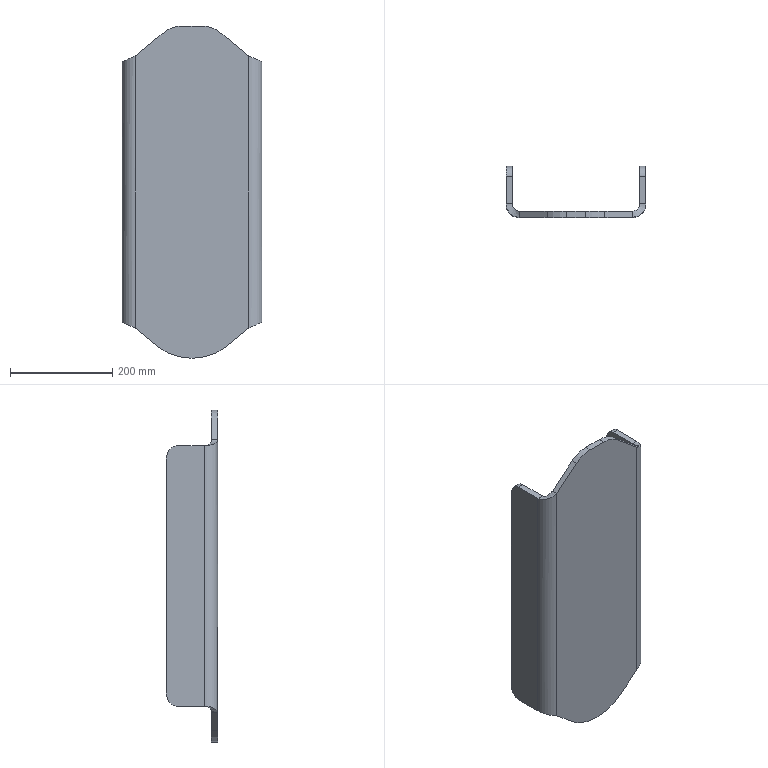Part | SolidWorks | features Fillet 3, Extrusion 1, FlatPattern 1, ICE 1, SheetMetal 1, SolidToSheetMetal 1 | 1 solid | 34 faces | box 274 x 100 x 650 mm | volume 2917891 mm3 | plane 18 | spline 8 | cylinder 8 | commonest cylinder face diameters 28 x2 52 x2 120 x2 200 x2
STEP:
#1=CARTESIAN_POINT('',(137.,-57.,579.897));
#2=VERTEX_POINT('',#1);
#3=CARTESIAN_POINT('',(125.,-57.,579.897));
#4=VERTEX_POINT('',#3);
#5=CARTESIAN_POINT('',(125.,-57.,579.897));
#6=DIRECTION('',(-1.,0.,0.));
#7=VECTOR('',#6,1000.);
#8=LINE('',#5,#7);
#9=EDGE_CURVE('',#2,#4,#8,.T.);
#10=ORIENTED_EDGE('',*,*,#9,.F.);
#11=CARTESIAN_POINT('',(137.,-37.,553.972));
#12=VERTEX_POINT('',#11);
#13=CARTESIAN_POINT('',(137.,-57.,579.897));
#14=CARTESIAN_POINT('',(137.,-45.284,579.897));
#15=CARTESIAN_POINT('',(137.,-37.,569.159));
#16=CARTESIAN_POINT('',(137.,-37.,553.972));
#17=(BOUNDED_CURVE()B_SPLINE_CURVE(3,(#13,#14,#15,#16),.UNSPECIFIED.,.F.,.F.)B_SPLINE_CURVE_WITH_KNOTS((4,4),(3.142,4.712),.UNSPECIFIED.)CURVE()GEOMETRIC_REPRESENTATION_ITEM()RATIONAL_B_SPLINE_CURVE((1.,0.8047,0.8047,1.))REPRESENTATION_ITEM(''));
#18=EDGE_CURVE('',#2,#12,#17,.T.);
#19=ORIENTED_EDGE('',*,*,#18,.T.);
#20=CARTESIAN_POINT('',(125.,-37.,553.972));
#21=VERTEX_POINT('',#20);
#22=CARTESIAN_POINT('',(125.,-37.,553.972));
#23=DIRECTION('',(-1.,0.,0.));
#24=VECTOR('',#23,1000.);
#25=LINE('',#22,#24);
#26=EDGE_CURVE('',#12,#21,#25,.T.);
#27=ORIENTED_EDGE('',*,*,#26,.T.);
#28=CARTESIAN_POINT('',(125.,-57.,579.897));
#29=CARTESIAN_POINT('',(125.,-45.284,579.897));
#30=CARTESIAN_POINT('',(125.,-37.,569.159));
#31=CARTESIAN_POINT('',(125.,-37.,553.972));
#32=(BOUNDED_CURVE()B_SPLINE_CURVE(3,(#28,#29,#30,#31),.UNSPECIFIED.,.F.,.T.)B_SPLINE_CURVE_WITH_KNOTS((4,4),(3.142,4.712),.UNSPECIFIED.)CURVE()GEOMETRIC_REPRESENTATION_ITEM()RATIONAL_B_SPLINE_CURVE((1.,0.8047,0.8047,1.))REPRESENTATION_ITEM(''));
#33=EDGE_CURVE('',#4,#21,#32,.T.);
#34=ORIENTED_EDGE('',*,*,#33,.F.);
#35=EDGE_LOOP('',(#10,#19,#27,#34));
#36=FACE_OUTER_BOUND('',#35,.T.);
#37=CARTESIAN_POINT('',(125.,-37.,553.972));
#38=CARTESIAN_POINT('',(137.,-37.,553.972));
#39=CARTESIAN_POINT('',(125.,-37.,569.159));
#40=CARTESIAN_POINT('',(137.,-37.,569.159));
#41=CARTESIAN_POINT('',(125.,-45.284,579.897));
#42=CARTESIAN_POINT('',(137.,-45.284,579.897));
#43=CARTESIAN_POINT('',(125.,-57.,579.897));
#44=CARTESIAN_POINT('',(137.,-57.,579.897));
#45=(BOUNDED_SURFACE()B_SPLINE_SURFACE(3,1,((#37,#38),(#39,#40),(#41,#42),(#43,#44)),.UNSPECIFIED.,.F.,.F.,.F.)B_SPLINE_SURFACE_WITH_KNOTS((4,4),(2,2),(0.,1.),(0.,1.),.UNSPECIFIED.)GEOMETRIC_REPRESENTATION_ITEM()RATIONAL_B_SPLINE_SURFACE(((1.,1.),(0.8047,0.8047),(0.8047,0.8047),(1.,1.)))REPRESENTATION_ITEM('')SURFACE());
#46=ADVANCED_FACE('',(#36),#45,.T.);
#47=ORIENTED_EDGE('',*,*,#26,.F.);
#48=CARTESIAN_POINT('',(137.,-37.,96.028));
#49=VERTEX_POINT('',#48);
#50=CARTESIAN_POINT('',(137.,-37.,650.));
#51=DIRECTION('',(0.,0.,-1.));
#52=VECTOR('',#51,1000.);
#53=LINE('',#50,#52);
#54=EDGE_CURVE('',#12,#49,#53,.T.);
#55=ORIENTED_EDGE('',*,*,#54,.T.);
#56=CARTESIAN_POINT('',(125.,-37.,96.028));
#57=VERTEX_POINT('',#56);
#58=CARTESIAN_POINT('',(125.,-37.,96.028));
#59=DIRECTION('',(-1.,0.,0.));
#60=VECTOR('',#59,1000.);
#61=LINE('',#58,#60);
#62=EDGE_CURVE('',#49,#57,#61,.T.);
#63=ORIENTED_EDGE('',*,*,#62,.T.);
#64=CARTESIAN_POINT('',(125.,-37.,650.));
#65=DIRECTION('',(0.,0.,-1.));
#66=VECTOR('',#65,1000.);
#67=LINE('',#64,#66);
#68=EDGE_CURVE('',#21,#57,#67,.T.);
#69=ORIENTED_EDGE('',*,*,#68,.F.);
#70=EDGE_LOOP('',(#47,#55,#63,#69));
#71=FACE_OUTER_BOUND('',#70,.T.);
#72=CARTESIAN_POINT('',(125.,-37.,650.));
#73=DIRECTION('',(0.,-1.,0.));
#74=DIRECTION('',(0.,0.,-1.));
#75=AXIS2_PLACEMENT_3D('',#72,#73,#74);
#76=PLANE('',#75);
#77=ADVANCED_FACE('',(#71),#76,.F.);
#78=ORIENTED_EDGE('',*,*,#62,.F.);
#79=CARTESIAN_POINT('',(137.,-57.,70.103));
#80=VERTEX_POINT('',#79);
#81=CARTESIAN_POINT('',(137.,-37.,96.028));
#82=CARTESIAN_POINT('',(137.,-37.,80.841));
#83=CARTESIAN_POINT('',(137.,-45.284,70.103));
#84=CARTESIAN_POINT('',(137.,-57.,70.103));
#85=(BOUNDED_CURVE()B_SPLINE_CURVE(3,(#81,#82,#83,#84),.UNSPECIFIED.,.F.,.F.)B_SPLINE_CURVE_WITH_KNOTS((4,4),(4.712,6.283),.UNSPECIFIED.)CURVE()GEOMETRIC_REPRESENTATION_ITEM()RATIONAL_B_SPLINE_CURVE((1.,0.8047,0.8047,1.))REPRESENTATION_ITEM(''));
#86=EDGE_CURVE('',#49,#80,#85,.T.);
#87=ORIENTED_EDGE('',*,*,#86,.T.);
#88=CARTESIAN_POINT('',(125.,-57.,70.103));
#89=VERTEX_POINT('',#88);
#90=CARTESIAN_POINT('',(125.,-57.,70.103));
#91=DIRECTION('',(-1.,0.,0.));
#92=VECTOR('',#91,1000.);
#93=LINE('',#90,#92);
#94=EDGE_CURVE('',#80,#89,#93,.T.);
#95=ORIENTED_EDGE('',*,*,#94,.T.);
#96=CARTESIAN_POINT('',(125.,-37.,96.028));
#97=CARTESIAN_POINT('',(125.,-37.,80.841));
#98=CARTESIAN_POINT('',(125.,-45.284,70.103));
#99=CARTESIAN_POINT('',(125.,-57.,70.103));
#100=(BOUNDED_CURVE()B_SPLINE_CURVE(3,(#96,#97,#98,#99),.UNSPECIFIED.,.F.,.T.)B_SPLINE_CURVE_WITH_KNOTS((4,4),(4.712,6.283),.UNSPECIFIED.)CURVE()GEOMETRIC_REPRESENTATION_ITEM()RATIONAL_B_SPLINE_CURVE((1.,0.8047,0.8047,1.))REPRESENTATION_ITEM(''));
#101=EDGE_CURVE('',#57,#89,#100,.T.);
#102=ORIENTED_EDGE('',*,*,#101,.F.);
#103=EDGE_LOOP('',(#78,#87,#95,#102));
#104=FACE_OUTER_BOUND('',#103,.T.);
#105=CARTESIAN_POINT('',(125.,-57.,70.103));
#106=CARTESIAN_POINT('',(137.,-57.,70.103));
#107=CARTESIAN_POINT('',(125.,-45.284,70.103));
#108=CARTESIAN_POINT('',(137.,-45.284,70.103));
#109=CARTESIAN_POINT('',(125.,-37.,80.841));
#110=CARTESIAN_POINT('',(137.,-37.,80.841));
#111=CARTESIAN_POINT('',(125.,-37.,96.028));
#112=CARTESIAN_POINT('',(137.,-37.,96.028));
#113=(BOUNDED_SURFACE()B_SPLINE_SURFACE(3,1,((#105,#106),(#107,#108),(#109,#110),(#111,#112)),.UNSPECIFIED.,.F.,.F.,.F.)B_SPLINE_SURFACE_WITH_KNOTS((4,4),(2,2),(0.,1.),(0.,1.),.UNSPECIFIED.)GEOMETRIC_REPRESENTATION_ITEM()RATIONAL_B_SPLINE_SURFACE(((1.,1.),(0.8047,0.8047),(0.8047,0.8047),(1.,1.)))REPRESENTATION_ITEM('')SURFACE());
#114=ADVANCED_FACE('',(#104),#113,.T.);
#115=ORIENTED_EDGE('',*,*,#94,.F.);
#116=CARTESIAN_POINT('',(137.,-111.,70.103));
#117=VERTEX_POINT('',#116);
#118=CARTESIAN_POINT('',(137.,-37.,70.103));
#119=DIRECTION('',(0.,-1.,0.));
#120=VECTOR('',#119,1000.);
#121=LINE('',#118,#120);
#122=EDGE_CURVE('',#80,#117,#121,.T.);
#123=ORIENTED_EDGE('',*,*,#122,.T.);
#124=CARTESIAN_POINT('',(125.,-111.,70.103));
#125=VERTEX_POINT('',#124);
#126=CARTESIAN_POINT('',(125.,-111.,70.103));
#127=DIRECTION('',(-1.,0.,0.));
#128=VECTOR('',#127,1000.);
#129=LINE('',#126,#128);
#130=EDGE_CURVE('',#117,#125,#129,.T.);
#131=ORIENTED_EDGE('',*,*,#130,.T.);
#132=CARTESIAN_POINT('',(125.,-37.,70.103));
#133=DIRECTION('',(0.,-1.,0.));
#134=VECTOR('',#133,1000.);
#135=LINE('',#132,#134);
#136=EDGE_CURVE('',#89,#125,#135,.T.);
#137=ORIENTED_EDGE('',*,*,#136,.F.);
#138=EDGE_LOOP('',(#115,#123,#131,#137));
#139=FACE_OUTER_BOUND('',#138,.T.);
#140=CARTESIAN_POINT('',(125.,-37.,70.103));
#141=DIRECTION('',(0.,0.,1.));
#142=DIRECTION('',(0.,-1.,0.));
#143=AXIS2_PLACEMENT_3D('',#140,#141,#142);
#144=PLANE('',#143);
#145=ADVANCED_FACE('',(#139),#144,.F.);
#146=ORIENTED_EDGE('',*,*,#130,.F.);
#147=CARTESIAN_POINT('',(111.,-137.,58.557));
#148=VERTEX_POINT('',#147);
#149=CARTESIAN_POINT('',(137.,-111.,70.103));
#150=CARTESIAN_POINT('',(137.,-126.23,70.103));
#151=CARTESIAN_POINT('',(126.23,-137.,65.32));
#152=CARTESIAN_POINT('',(111.,-137.,58.557));
#153=(BOUNDED_CURVE()B_SPLINE_CURVE(3,(#149,#150,#151,#152),.UNSPECIFIED.,.F.,.F.)B_SPLINE_CURVE_WITH_KNOTS((4,4),(3.142,4.712),.UNSPECIFIED.)CURVE()GEOMETRIC_REPRESENTATION_ITEM()RATIONAL_B_SPLINE_CURVE((1.,0.8047,0.8047,1.))REPRESENTATION_ITEM(''));
#154=EDGE_CURVE('',#117,#148,#153,.T.);
#155=ORIENTED_EDGE('',*,*,#154,.T.);
#156=CARTESIAN_POINT('',(111.,-125.,58.557));
#157=VERTEX_POINT('',#156);
#158=CARTESIAN_POINT('',(111.,-125.,58.557));
#159=DIRECTION('',(0.,1.,0.));
#160=VECTOR('',#159,1000.);
#161=LINE('',#158,#160);
#162=EDGE_CURVE('',#148,#157,#161,.T.);
#163=ORIENTED_EDGE('',*,*,#162,.T.);
#164=CARTESIAN_POINT('',(125.,-111.,70.103));
#165=CARTESIAN_POINT('',(125.,-119.201,70.103));
#166=CARTESIAN_POINT('',(119.201,-125.,65.32));
#167=CARTESIAN_POINT('',(111.,-125.,58.557));
#168=(BOUNDED_CURVE()B_SPLINE_CURVE(3,(#164,#165,#166,#167),.UNSPECIFIED.,.F.,.F.)B_SPLINE_CURVE_WITH_KNOTS((4,4),(3.142,4.712),.UNSPECIFIED.)CURVE()GEOMETRIC_REPRESENTATION_ITEM()RATIONAL_B_SPLINE_CURVE((1.,0.8047,0.8047,1.))REPRESENTATION_ITEM(''));
#169=EDGE_CURVE('',#125,#157,#168,.T.);
#170=ORIENTED_EDGE('',*,*,#169,.F.);
#171=EDGE_LOOP('',(#146,#155,#163,#170));
#172=FACE_OUTER_BOUND('',#171,.T.);
#173=CARTESIAN_POINT('',(85.,-111.,47.01));
#174=CARTESIAN_POINT('',(89.,-111.,47.01));
#175=CARTESIAN_POINT('',(93.,-111.,47.01));
#176=CARTESIAN_POINT('',(97.,-111.,47.01));
#177=CARTESIAN_POINT('',(85.,-59.,47.01));
#178=CARTESIAN_POINT('',(89.,-67.,47.01));
#179=CARTESIAN_POINT('',(93.,-75.,47.01));
#180=CARTESIAN_POINT('',(97.,-83.,47.01));
#181=CARTESIAN_POINT('',(137.,-59.,70.103));
#182=CARTESIAN_POINT('',(133.,-67.,70.103));
#183=CARTESIAN_POINT('',(129.,-75.,70.103));
#184=CARTESIAN_POINT('',(125.,-83.,70.103));
#185=CARTESIAN_POINT('',(137.,-111.,70.103));
#186=CARTESIAN_POINT('',(133.,-111.,70.103));
#187=CARTESIAN_POINT('',(129.,-111.,70.103));
#188=CARTESIAN_POINT('',(125.,-111.,70.103));
#189=CARTESIAN_POINT('',(137.,-163.,70.103));
#190=CARTESIAN_POINT('',(133.,-155.,70.103));
#191=CARTESIAN_POINT('',(129.,-147.,70.103));
#192=CARTESIAN_POINT('',(125.,-139.,70.103));
#193=CARTESIAN_POINT('',(85.,-163.,47.01));
#194=CARTESIAN_POINT('',(89.,-155.,47.01));
#195=CARTESIAN_POINT('',(93.,-147.,47.01));
#196=CARTESIAN_POINT('',(97.,-139.,47.01));
#197=CARTESIAN_POINT('',(85.,-111.,47.01));
#198=CARTESIAN_POINT('',(89.,-111.,47.01));
#199=CARTESIAN_POINT('',(93.,-111.,47.01));
#200=CARTESIAN_POINT('',(97.,-111.,47.01));
#201=(BOUNDED_SURFACE()B_SPLINE_SURFACE(3,3,((#173,#174,#175,#176),(#177,#178,#179,#180),(#181,#182,#183,#184),(#185,#186,#187,#188),(#189,#190,#191,#192),(#193,#194,#195,#196),(#197,#198,#199,#200)),.UNSPECIFIED.,.T.,.F.,.F.)B_SPLINE_SURFACE_WITH_KNOTS((4,3,4),(4,4),(0.,0.5,1.),(0.,1.),.UNSPECIFIED.)GEOMETRIC_REPRESENTATION_ITEM()RATIONAL_B_SPLINE_SURFACE(((1.,1.,1.,1.),(0.3333,0.3333,0.3333,0.3333),(0.3333,0.3333,0.3333,0.3333),(1.,1.,1.,1.),(0.3333,0.3333,0.3333,0.3333),(0.3333,0.3333,0.3333,0.3333),(1.,1.,1.,1.)))REPRESENTATION_ITEM('')SURFACE());
#202=ADVANCED_FACE('',(#172),#201,.T.);
#203=ORIENTED_EDGE('',*,*,#162,.F.);
#204=CARTESIAN_POINT('',(67.709,-137.,22.853));
#205=VERTEX_POINT('',#204);
#206=CARTESIAN_POINT('',(269.189,-137.,189.021));
#207=DIRECTION('',(-0.7715,0.,-0.6363));
#208=VECTOR('',#207,1000.);
#209=LINE('',#206,#208);
#210=EDGE_CURVE('',#148,#205,#209,.T.);
#211=ORIENTED_EDGE('',*,*,#210,.T.);
#212=CARTESIAN_POINT('',(67.709,-125.,22.853));
#213=VERTEX_POINT('',#212);
#214=CARTESIAN_POINT('',(67.709,-125.,22.853));
#215=DIRECTION('',(0.,1.,0.));
#216=VECTOR('',#215,1000.);
#217=LINE('',#214,#216);
#218=EDGE_CURVE('',#205,#213,#217,.T.);
#219=ORIENTED_EDGE('',*,*,#218,.T.);
#220=CARTESIAN_POINT('',(269.189,-125.,189.021));
#221=DIRECTION('',(-0.7715,0.,-0.6363));
#222=VECTOR('',#221,1000.);
#223=LINE('',#220,#222);
#224=EDGE_CURVE('',#157,#213,#223,.T.);
#225=ORIENTED_EDGE('',*,*,#224,.F.);
#226=EDGE_LOOP('',(#203,#211,#219,#225));
#227=FACE_OUTER_BOUND('',#226,.T.);
#228=CARTESIAN_POINT('',(269.189,-125.,189.021));
#229=DIRECTION('',(-0.6363,0.,0.7715));
#230=DIRECTION('',(-0.7715,0.,-0.6363));
#231=AXIS2_PLACEMENT_3D('',#228,#229,#230);
#232=PLANE('',#231);
#233=ADVANCED_FACE('',(#227),#232,.F.);
#234=ORIENTED_EDGE('',*,*,#218,.F.);
#235=CARTESIAN_POINT('',(4.083,-137.,0.));
#236=VERTEX_POINT('',#235);
#237=CARTESIAN_POINT('',(4.083,-137.,100.));
#238=DIRECTION('',(0.,1.,0.));
#239=DIRECTION('',(1.,0.,0.));
#240=AXIS2_PLACEMENT_3D('',#237,#238,#239);
#241=CIRCLE('',#240,100.);
#242=EDGE_CURVE('',#205,#236,#241,.T.);
#243=ORIENTED_EDGE('',*,*,#242,.T.);
#244=CARTESIAN_POINT('',(4.083,-125.,0.));
#245=VERTEX_POINT('',#244);
#246=CARTESIAN_POINT('',(4.083,-125.,0.));
#247=DIRECTION('',(0.,1.,0.));
#248=VECTOR('',#247,1000.);
#249=LINE('',#246,#248);
#250=EDGE_CURVE('',#236,#245,#249,.T.);
#251=ORIENTED_EDGE('',*,*,#250,.T.);
#252=CARTESIAN_POINT('',(4.083,-125.,100.));
#253=DIRECTION('',(0.,1.,0.));
#254=DIRECTION('',(1.,0.,0.));
#255=AXIS2_PLACEMENT_3D('',#252,#253,#254);
#256=CIRCLE('',#255,100.);
#257=EDGE_CURVE('',#213,#245,#256,.T.);
#258=ORIENTED_EDGE('',*,*,#257,.F.);
#259=EDGE_LOOP('',(#234,#243,#251,#258));
#260=FACE_OUTER_BOUND('',#259,.T.);
#261=CARTESIAN_POINT('',(4.083,-125.,100.));
#262=DIRECTION('',(0.,-1.,0.));
#263=DIRECTION('',(1.,0.,0.));
#264=AXIS2_PLACEMENT_3D('',#261,#262,#263);
#265=CYLINDRICAL_SURFACE('',#264,100.);
#266=ADVANCED_FACE('',(#260),#265,.T.);
#267=ORIENTED_EDGE('',*,*,#250,.F.);
#268=CARTESIAN_POINT('',(-4.083,-137.,0.));
#269=VERTEX_POINT('',#268);
#270=CARTESIAN_POINT('',(-111.,-137.,0.));
#271=DIRECTION('',(-1.,0.,0.));
#272=VECTOR('',#271,1000.);
#273=LINE('',#270,#272);
#274=EDGE_CURVE('',#236,#269,#273,.T.);
#275=ORIENTED_EDGE('',*,*,#274,.T.);
#276=CARTESIAN_POINT('',(-4.083,-125.,0.));
#277=VERTEX_POINT('',#276);
#278=CARTESIAN_POINT('',(-4.083,-125.,0.));
#279=DIRECTION('',(0.,1.,0.));
#280=VECTOR('',#279,1000.);
#281=LINE('',#278,#280);
#282=EDGE_CURVE('',#269,#277,#281,.T.);
#283=ORIENTED_EDGE('',*,*,#282,.T.);
#284=CARTESIAN_POINT('',(-111.,-125.,0.));
#285=DIRECTION('',(-1.,0.,0.));
#286=VECTOR('',#285,1000.);
#287=LINE('',#284,#286);
#288=EDGE_CURVE('',#245,#277,#287,.T.);
#289=ORIENTED_EDGE('',*,*,#288,.F.);
#290=EDGE_LOOP('',(#267,#275,#283,#289));
#291=FACE_OUTER_BOUND('',#290,.T.);
#292=CARTESIAN_POINT('',(-111.,-125.,0.));
#293=DIRECTION('',(0.,0.,1.));
#294=DIRECTION('',(-1.,0.,0.));
#295=AXIS2_PLACEMENT_3D('',#292,#293,#294);
#296=PLANE('',#295);
#297=ADVANCED_FACE('',(#291),#296,.F.);
#298=ORIENTED_EDGE('',*,*,#282,.F.);
#299=CARTESIAN_POINT('',(-67.709,-137.,22.853));
#300=VERTEX_POINT('',#299);
#301=CARTESIAN_POINT('',(-4.083,-137.,100.));
#302=DIRECTION('',(0.,1.,0.));
#303=DIRECTION('',(1.,0.,0.));
#304=AXIS2_PLACEMENT_3D('',#301,#302,#303);
#305=CIRCLE('',#304,100.);
#306=EDGE_CURVE('',#269,#300,#305,.T.);
#307=ORIENTED_EDGE('',*,*,#306,.T.);
#308=CARTESIAN_POINT('',(-67.709,-125.,22.853));
#309=VERTEX_POINT('',#308);
#310=CARTESIAN_POINT('',(-67.709,-125.,22.853));
#311=DIRECTION('',(0.,1.,0.));
#312=VECTOR('',#311,1000.);
#313=LINE('',#310,#312);
#314=EDGE_CURVE('',#300,#309,#313,.T.);
#315=ORIENTED_EDGE('',*,*,#314,.T.);
#316=CARTESIAN_POINT('',(-4.083,-125.,100.));
#317=DIRECTION('',(0.,1.,0.));
#318=DIRECTION('',(1.,0.,0.));
#319=AXIS2_PLACEMENT_3D('',#316,#317,#318);
#320=CIRCLE('',#319,100.);
#321=EDGE_CURVE('',#277,#309,#320,.T.);
#322=ORIENTED_EDGE('',*,*,#321,.F.);
#323=EDGE_LOOP('',(#298,#307,#315,#322));
#324=FACE_OUTER_BOUND('',#323,.T.);
#325=CARTESIAN_POINT('',(-4.083,-125.,100.));
#326=DIRECTION('',(0.,-1.,0.));
#327=DIRECTION('',(1.,0.,0.));
#328=AXIS2_PLACEMENT_3D('',#325,#326,#327);
#329=CYLINDRICAL_SURFACE('',#328,100.);
#330=ADVANCED_FACE('',(#324),#329,.T.);
#331=ORIENTED_EDGE('',*,*,#314,.F.);
#332=CARTESIAN_POINT('',(-111.,-137.,58.557));
#333=VERTEX_POINT('',#332);
#334=CARTESIAN_POINT('',(-401.316,-137.,297.992));
#335=DIRECTION('',(-0.7715,0.,0.6363));
#336=VECTOR('',#335,1000.);
#337=LINE('',#334,#336);
#338=EDGE_CURVE('',#300,#333,#337,.T.);
#339=ORIENTED_EDGE('',*,*,#338,.T.);
#340=CARTESIAN_POINT('',(-111.,-125.,58.557));
#341=VERTEX_POINT('',#340);
#342=CARTESIAN_POINT('',(-111.,-125.,58.557));
#343=DIRECTION('',(0.,1.,0.));
#344=VECTOR('',#343,1000.);
#345=LINE('',#342,#344);
#346=EDGE_CURVE('',#333,#341,#345,.T.);
#347=ORIENTED_EDGE('',*,*,#346,.T.);
#348=CARTESIAN_POINT('',(-401.316,-125.,297.992));
#349=DIRECTION('',(-0.7715,0.,0.6363));
#350=VECTOR('',#349,1000.);
#351=LINE('',#348,#350);
#352=EDGE_CURVE('',#309,#341,#351,.T.);
#353=ORIENTED_EDGE('',*,*,#352,.F.);
#354=EDGE_LOOP('',(#331,#339,#347,#353));
#355=FACE_OUTER_BOUND('',#354,.T.);
#356=CARTESIAN_POINT('',(-401.316,-125.,297.992));
#357=DIRECTION('',(0.6363,0.,0.7715));
#358=DIRECTION('',(-0.7715,0.,0.6363));
#359=AXIS2_PLACEMENT_3D('',#356,#357,#358);
#360=PLANE('',#359);
#361=ADVANCED_FACE('',(#355),#360,.F.);
#362=ORIENTED_EDGE('',*,*,#346,.F.);
#363=CARTESIAN_POINT('',(-137.,-111.,70.103));
#364=VERTEX_POINT('',#363);
#365=CARTESIAN_POINT('',(-111.,-137.,58.557));
#366=CARTESIAN_POINT('',(-126.23,-137.,65.32));
#367=CARTESIAN_POINT('',(-137.,-126.23,70.103));
#368=CARTESIAN_POINT('',(-137.,-111.,70.103));
#369=(BOUNDED_CURVE()B_SPLINE_CURVE(3,(#365,#366,#367,#368),.UNSPECIFIED.,.F.,.T.)B_SPLINE_CURVE_WITH_KNOTS((4,4),(1.571,3.142),.UNSPECIFIED.)CURVE()GEOMETRIC_REPRESENTATION_ITEM()RATIONAL_B_SPLINE_CURVE((1.,0.8047,0.8047,1.))REPRESENTATION_ITEM(''));
#370=EDGE_CURVE('',#333,#364,#369,.T.);
#371=ORIENTED_EDGE('',*,*,#370,.T.);
#372=CARTESIAN_POINT('',(-125.,-111.,70.103));
#373=VERTEX_POINT('',#372);
#374=CARTESIAN_POINT('',(-125.,-111.,70.103));
#375=DIRECTION('',(1.,0.,0.));
#376=VECTOR('',#375,1000.);
#377=LINE('',#374,#376);
#378=EDGE_CURVE('',#364,#373,#377,.T.);
#379=ORIENTED_EDGE('',*,*,#378,.T.);
#380=CARTESIAN_POINT('',(-111.,-125.,58.557));
#381=CARTESIAN_POINT('',(-119.201,-125.,65.32));
#382=CARTESIAN_POINT('',(-125.,-119.201,70.103));
#383=CARTESIAN_POINT('',(-125.,-111.,70.103));
#384=(BOUNDED_CURVE()B_SPLINE_CURVE(3,(#380,#381,#382,#383),.UNSPECIFIED.,.F.,.T.)B_SPLINE_CURVE_WITH_KNOTS((4,4),(1.571,3.142),.UNSPECIFIED.)CURVE()GEOMETRIC_REPRESENTATION_ITEM()RATIONAL_B_SPLINE_CURVE((1.,0.8047,0.8047,1.))REPRESENTATION_ITEM(''));
#385=EDGE_CURVE('',#341,#373,#384,.T.);
#386=ORIENTED_EDGE('',*,*,#385,.F.);
#387=EDGE_LOOP('',(#362,#371,#379,#386));
#388=FACE_OUTER_BOUND('',#387,.T.);
#389=CARTESIAN_POINT('',(-85.,-111.,47.01));
#390=CARTESIAN_POINT('',(-89.,-111.,47.01));
#391=CARTESIAN_POINT('',(-93.,-111.,47.01));
#392=CARTESIAN_POINT('',(-97.,-111.,47.01));
#393=CARTESIAN_POINT('',(-85.,-163.,47.01));
#394=CARTESIAN_POINT('',(-89.,-155.,47.01));
#395=CARTESIAN_POINT('',(-93.,-147.,47.01));
#396=CARTESIAN_POINT('',(-97.,-139.,47.01));
#397=CARTESIAN_POINT('',(-137.,-163.,70.103));
#398=CARTESIAN_POINT('',(-133.,-155.,70.103));
#399=CARTESIAN_POINT('',(-129.,-147.,70.103));
#400=CARTESIAN_POINT('',(-125.,-139.,70.103));
#401=CARTESIAN_POINT('',(-137.,-111.,70.103));
#402=CARTESIAN_POINT('',(-133.,-111.,70.103));
#403=CARTESIAN_POINT('',(-129.,-111.,70.103));
#404=CARTESIAN_POINT('',(-125.,-111.,70.103));
#405=CARTESIAN_POINT('',(-137.,-59.,70.103));
#406=CARTESIAN_POINT('',(-133.,-67.,70.103));
#407=CARTESIAN_POINT('',(-129.,-75.,70.103));
#408=CARTESIAN_POINT('',(-125.,-83.,70.103));
#409=CARTESIAN_POINT('',(-85.,-59.,47.01));
#410=CARTESIAN_POINT('',(-89.,-67.,47.01));
#411=CARTESIAN_POINT('',(-93.,-75.,47.01));
#412=CARTESIAN_POINT('',(-97.,-83.,47.01));
#413=CARTESIAN_POINT('',(-85.,-111.,47.01));
#414=CARTESIAN_POINT('',(-89.,-111.,47.01));
#415=CARTESIAN_POINT('',(-93.,-111.,47.01));
#416=CARTESIAN_POINT('',(-97.,-111.,47.01));
#417=(BOUNDED_SURFACE()B_SPLINE_SURFACE(3,3,((#389,#390,#391,#392),(#393,#394,#395,#396),(#397,#398,#399,#400),(#401,#402,#403,#404),(#405,#406,#407,#408),(#409,#410,#411,#412),(#413,#414,#415,#416)),.UNSPECIFIED.,.T.,.F.,.F.)B_SPLINE_SURFACE_WITH_KNOTS((4,3,4),(4,4),(0.,0.5,1.),(0.,1.),.UNSPECIFIED.)GEOMETRIC_REPRESENTATION_ITEM()RATIONAL_B_SPLINE_SURFACE(((1.,1.,1.,1.),(0.3333,0.3333,0.3333,0.3333),(0.3333,0.3333,0.3333,0.3333),(1.,1.,1.,1.),(0.3333,0.3333,0.3333,0.3333),(0.3333,0.3333,0.3333,0.3333),(1.,1.,1.,1.)))REPRESENTATION_ITEM('')SURFACE());
#418=ADVANCED_FACE('',(#388),#417,.T.);
#419=ORIENTED_EDGE('',*,*,#378,.F.);
#420=CARTESIAN_POINT('',(-137.,-57.,70.103));
#421=VERTEX_POINT('',#420);
#422=CARTESIAN_POINT('',(-137.,-37.,70.103));
#423=DIRECTION('',(0.,1.,0.));
#424=VECTOR('',#423,1000.);
#425=LINE('',#422,#424);
#426=EDGE_CURVE('',#364,#421,#425,.T.);
#427=ORIENTED_EDGE('',*,*,#426,.T.);
#428=CARTESIAN_POINT('',(-125.,-57.,70.103));
#429=VERTEX_POINT('',#428);
#430=CARTESIAN_POINT('',(-125.,-57.,70.103));
#431=DIRECTION('',(1.,0.,0.));
#432=VECTOR('',#431,1000.);
#433=LINE('',#430,#432);
#434=EDGE_CURVE('',#421,#429,#433,.T.);
#435=ORIENTED_EDGE('',*,*,#434,.T.);
#436=CARTESIAN_POINT('',(-125.,-37.,70.103));
#437=DIRECTION('',(0.,1.,0.));
#438=VECTOR('',#437,1000.);
#439=LINE('',#436,#438);
#440=EDGE_CURVE('',#373,#429,#439,.T.);
#441=ORIENTED_EDGE('',*,*,#440,.F.);
#442=EDGE_LOOP('',(#419,#427,#435,#441));
#443=FACE_OUTER_BOUND('',#442,.T.);
#444=CARTESIAN_POINT('',(-125.,-37.,70.103));
#445=DIRECTION('',(0.,0.,1.));
#446=DIRECTION('',(0.,1.,0.));
#447=AXIS2_PLACEMENT_3D('',#444,#445,#446);
#448=PLANE('',#447);
#449=ADVANCED_FACE('',(#443),#448,.F.);
#450=ORIENTED_EDGE('',*,*,#434,.F.);
#451=CARTESIAN_POINT('',(-137.,-37.,96.028));
#452=VERTEX_POINT('',#451);
#453=CARTESIAN_POINT('',(-137.,-57.,70.103));
#454=CARTESIAN_POINT('',(-137.,-45.284,70.103));
#455=CARTESIAN_POINT('',(-137.,-37.,80.841));
#456=CARTESIAN_POINT('',(-137.,-37.,96.028));
#457=(BOUNDED_CURVE()B_SPLINE_CURVE(3,(#453,#454,#455,#456),.UNSPECIFIED.,.F.,.T.)B_SPLINE_CURVE_WITH_KNOTS((4,4),(3.142,4.712),.UNSPECIFIED.)CURVE()GEOMETRIC_REPRESENTATION_ITEM()RATIONAL_B_SPLINE_CURVE((1.,0.8047,0.8047,1.))REPRESENTATION_ITEM(''));
#458=EDGE_CURVE('',#421,#452,#457,.T.);
#459=ORIENTED_EDGE('',*,*,#458,.T.);
#460=CARTESIAN_POINT('',(-125.,-37.,96.028));
#461=VERTEX_POINT('',#460);
#462=CARTESIAN_POINT('',(-125.,-37.,96.028));
#463=DIRECTION('',(1.,0.,0.));
#464=VECTOR('',#463,1000.);
#465=LINE('',#462,#464);
#466=EDGE_CURVE('',#452,#461,#465,.T.);
#467=ORIENTED_EDGE('',*,*,#466,.T.);
#468=CARTESIAN_POINT('',(-125.,-57.,70.103));
#469=CARTESIAN_POINT('',(-125.,-45.284,70.103));
#470=CARTESIAN_POINT('',(-125.,-37.,80.841));
#471=CARTESIAN_POINT('',(-125.,-37.,96.028));
#472=(BOUNDED_CURVE()B_SPLINE_CURVE(3,(#468,#469,#470,#471),.UNSPECIFIED.,.F.,.F.)B_SPLINE_CURVE_WITH_KNOTS((4,4),(3.142,4.712),.UNSPECIFIED.)CURVE()GEOMETRIC_REPRESENTATION_ITEM()RATIONAL_B_SPLINE_CURVE((1.,0.8047,0.8047,1.))REPRESENTATION_ITEM(''));
#473=EDGE_CURVE('',#429,#461,#472,.T.);
#474=ORIENTED_EDGE('',*,*,#473,.F.);
#475=EDGE_LOOP('',(#450,#459,#467,#474));
#476=FACE_OUTER_BOUND('',#475,.T.);
#477=CARTESIAN_POINT('',(-125.,-37.,96.028));
#478=CARTESIAN_POINT('',(-137.,-37.,96.028));
#479=CARTESIAN_POINT('',(-125.,-37.,80.841));
#480=CARTESIAN_POINT('',(-137.,-37.,80.841));
#481=CARTESIAN_POINT('',(-125.,-45.284,70.103));
#482=CARTESIAN_POINT('',(-137.,-45.284,70.103));
#483=CARTESIAN_POINT('',(-125.,-57.,70.103));
#484=CARTESIAN_POINT('',(-137.,-57.,70.103));
#485=(BOUNDED_SURFACE()B_SPLINE_SURFACE(3,1,((#477,#478),(#479,#480),(#481,#482),(#483,#484)),.UNSPECIFIED.,.F.,.F.,.F.)B_SPLINE_SURFACE_WITH_KNOTS((4,4),(2,2),(0.,1.),(0.,1.),.UNSPECIFIED.)GEOMETRIC_REPRESENTATION_ITEM()RATIONAL_B_SPLINE_SURFACE(((1.,1.),(0.8047,0.8047),(0.8047,0.8047),(1.,1.)))REPRESENTATION_ITEM('')SURFACE());
#486=ADVANCED_FACE('',(#476),#485,.T.);
#487=ORIENTED_EDGE('',*,*,#466,.F.);
#488=CARTESIAN_POINT('',(-137.,-37.,553.972));
#489=VERTEX_POINT('',#488);
#490=CARTESIAN_POINT('',(-137.,-37.,650.));
#491=DIRECTION('',(0.,0.,-1.));
#492=VECTOR('',#491,1000.);
#493=LINE('',#490,#492);
#494=EDGE_CURVE('',#489,#452,#493,.T.);
#495=ORIENTED_EDGE('',*,*,#494,.F.);
#496=CARTESIAN_POINT('',(-125.,-37.,553.972));
#497=VERTEX_POINT('',#496);
#498=CARTESIAN_POINT('',(-125.,-37.,553.972));
#499=DIRECTION('',(1.,0.,0.));
#500=VECTOR('',#499,1000.);
#501=LINE('',#498,#500);
#502=EDGE_CURVE('',#489,#497,#501,.T.);
#503=ORIENTED_EDGE('',*,*,#502,.T.);
#504=CARTESIAN_POINT('',(-125.,-37.,650.));
#505=DIRECTION('',(0.,0.,-1.));
#506=VECTOR('',#505,1000.);
#507=LINE('',#504,#506);
#508=EDGE_CURVE('',#497,#461,#507,.T.);
#509=ORIENTED_EDGE('',*,*,#508,.T.);
#510=EDGE_LOOP('',(#487,#495,#503,#509));
#511=FACE_OUTER_BOUND('',#510,.T.);
#512=CARTESIAN_POINT('',(-125.,-37.,650.));
#513=DIRECTION('',(0.,1.,0.));
#514=DIRECTION('',(0.,0.,-1.));
#515=AXIS2_PLACEMENT_3D('',#512,#513,#514);
#516=PLANE('',#515);
#517=ADVANCED_FACE('',(#511),#516,.T.);
#518=ORIENTED_EDGE('',*,*,#502,.F.);
#519=CARTESIAN_POINT('',(-137.,-57.,579.897));
#520=VERTEX_POINT('',#519);
#521=CARTESIAN_POINT('',(-137.,-37.,553.972));
#522=CARTESIAN_POINT('',(-137.,-37.,569.159));
#523=CARTESIAN_POINT('',(-137.,-45.284,579.897));
#524=CARTESIAN_POINT('',(-137.,-57.,579.897));
#525=(BOUNDED_CURVE()B_SPLINE_CURVE(3,(#521,#522,#523,#524),.UNSPECIFIED.,.F.,.T.)B_SPLINE_CURVE_WITH_KNOTS((4,4),(4.712,6.283),.UNSPECIFIED.)CURVE()GEOMETRIC_REPRESENTATION_ITEM()RATIONAL_B_SPLINE_CURVE((1.,0.8047,0.8047,1.))REPRESENTATION_ITEM(''));
#526=EDGE_CURVE('',#489,#520,#525,.T.);
#527=ORIENTED_EDGE('',*,*,#526,.T.);
#528=CARTESIAN_POINT('',(-125.,-57.,579.897));
#529=VERTEX_POINT('',#528);
#530=CARTESIAN_POINT('',(-125.,-57.,579.897));
#531=DIRECTION('',(1.,0.,0.));
#532=VECTOR('',#531,1000.);
#533=LINE('',#530,#532);
#534=EDGE_CURVE('',#520,#529,#533,.T.);
#535=ORIENTED_EDGE('',*,*,#534,.T.);
#536=CARTESIAN_POINT('',(-125.,-37.,553.972));
#537=CARTESIAN_POINT('',(-125.,-37.,569.159));
#538=CARTESIAN_POINT('',(-125.,-45.284,579.897));
#539=CARTESIAN_POINT('',(-125.,-57.,579.897));
#540=(BOUNDED_CURVE()B_SPLINE_CURVE(3,(#536,#537,#538,#539),.UNSPECIFIED.,.F.,.T.)B_SPLINE_CURVE_WITH_KNOTS((4,4),(4.712,6.283),.UNSPECIFIED.)CURVE()GEOMETRIC_REPRESENTATION_ITEM()RATIONAL_B_SPLINE_CURVE((1.,0.8047,0.8047,1.))REPRESENTATION_ITEM(''));
#541=EDGE_CURVE('',#497,#529,#540,.T.);
#542=ORIENTED_EDGE('',*,*,#541,.F.);
#543=EDGE_LOOP('',(#518,#527,#535,#542));
#544=FACE_OUTER_BOUND('',#543,.T.);
#545=CARTESIAN_POINT('',(-125.,-57.,579.897));
#546=CARTESIAN_POINT('',(-137.,-57.,579.897));
#547=CARTESIAN_POINT('',(-125.,-45.284,579.897));
#548=CARTESIAN_POINT('',(-137.,-45.284,579.897));
#549=CARTESIAN_POINT('',(-125.,-37.,569.159));
#550=CARTESIAN_POINT('',(-137.,-37.,569.159));
#551=CARTESIAN_POINT('',(-125.,-37.,553.972));
#552=CARTESIAN_POINT('',(-137.,-37.,553.972));
#553=(BOUNDED_SURFACE()B_SPLINE_SURFACE(3,1,((#545,#546),(#547,#548),(#549,#550),(#551,#552)),.UNSPECIFIED.,.F.,.F.,.F.)B_SPLINE_SURFACE_WITH_KNOTS((4,4),(2,2),(0.,1.),(0.,1.),.UNSPECIFIED.)GEOMETRIC_REPRESENTATION_ITEM()RATIONAL_B_SPLINE_SURFACE(((1.,1.),(0.8047,0.8047),(0.8047,0.8047),(1.,1.)))REPRESENTATION_ITEM('')SURFACE());
#554=ADVANCED_FACE('',(#544),#553,.T.);
#555=ORIENTED_EDGE('',*,*,#534,.F.);
#556=CARTESIAN_POINT('',(-137.,-111.,579.897));
#557=VERTEX_POINT('',#556);
#558=CARTESIAN_POINT('',(-137.,-37.,579.897));
#559=DIRECTION('',(0.,-1.,0.));
#560=VECTOR('',#559,1000.);
#561=LINE('',#558,#560);
#562=EDGE_CURVE('',#520,#557,#561,.T.);
#563=ORIENTED_EDGE('',*,*,#562,.T.);
#564=CARTESIAN_POINT('',(-125.,-111.,579.897));
#565=VERTEX_POINT('',#564);
#566=CARTESIAN_POINT('',(-125.,-111.,579.897));
#567=DIRECTION('',(1.,0.,0.));
#568=VECTOR('',#567,1000.);
#569=LINE('',#566,#568);
#570=EDGE_CURVE('',#557,#565,#569,.T.);
#571=ORIENTED_EDGE('',*,*,#570,.T.);
#572=CARTESIAN_POINT('',(-125.,-37.,579.897));
#573=DIRECTION('',(0.,-1.,0.));
#574=VECTOR('',#573,1000.);
#575=LINE('',#572,#574);
#576=EDGE_CURVE('',#529,#565,#575,.T.);
#577=ORIENTED_EDGE('',*,*,#576,.F.);
#578=EDGE_LOOP('',(#555,#563,#571,#577));
#579=FACE_OUTER_BOUND('',#578,.T.);
#580=CARTESIAN_POINT('',(-125.,-37.,579.897));
#581=DIRECTION('',(0.,0.,-1.));
#582=DIRECTION('',(0.,-1.,0.));
#583=AXIS2_PLACEMENT_3D('',#580,#581,#582);
#584=PLANE('',#583);
#585=ADVANCED_FACE('',(#579),#584,.F.);
#586=ORIENTED_EDGE('',*,*,#570,.F.);
#587=CARTESIAN_POINT('',(-111.,-137.,591.443));
#588=VERTEX_POINT('',#587);
#589=CARTESIAN_POINT('',(-137.,-111.,579.897));
#590=CARTESIAN_POINT('',(-137.,-126.23,579.897));
#591=CARTESIAN_POINT('',(-126.23,-137.,584.68));
#592=CARTESIAN_POINT('',(-111.,-137.,591.443));
#593=(BOUNDED_CURVE()B_SPLINE_CURVE(3,(#589,#590,#591,#592),.UNSPECIFIED.,.F.,.F.)B_SPLINE_CURVE_WITH_KNOTS((4,4),(0.,1.571),.UNSPECIFIED.)CURVE()GEOMETRIC_REPRESENTATION_ITEM()RATIONAL_B_SPLINE_CURVE((1.,0.8047,0.8047,1.))REPRESENTATION_ITEM(''));
#594=EDGE_CURVE('',#557,#588,#593,.T.);
#595=ORIENTED_EDGE('',*,*,#594,.T.);
#596=CARTESIAN_POINT('',(-111.,-125.,591.443));
#597=VERTEX_POINT('',#596);
#598=CARTESIAN_POINT('',(-111.,-125.,591.443));
#599=DIRECTION('',(0.,1.,0.));
#600=VECTOR('',#599,1000.);
#601=LINE('',#598,#600);
#602=EDGE_CURVE('',#588,#597,#601,.T.);
#603=ORIENTED_EDGE('',*,*,#602,.T.);
#604=CARTESIAN_POINT('',(-125.,-111.,579.897));
#605=CARTESIAN_POINT('',(-125.,-119.201,579.897));
#606=CARTESIAN_POINT('',(-119.201,-125.,584.68));
#607=CARTESIAN_POINT('',(-111.,-125.,591.443));
#608=(BOUNDED_CURVE()B_SPLINE_CURVE(3,(#604,#605,#606,#607),.UNSPECIFIED.,.F.,.F.)B_SPLINE_CURVE_WITH_KNOTS((4,4),(0.,1.571),.UNSPECIFIED.)CURVE()GEOMETRIC_REPRESENTATION_ITEM()RATIONAL_B_SPLINE_CURVE((1.,0.8047,0.8047,1.))REPRESENTATION_ITEM(''));
#609=EDGE_CURVE('',#565,#597,#608,.T.);
#610=ORIENTED_EDGE('',*,*,#609,.F.);
#611=EDGE_LOOP('',(#586,#595,#603,#610));
#612=FACE_OUTER_BOUND('',#611,.T.);
#613=CARTESIAN_POINT('',(-137.,-111.,579.897));
#614=CARTESIAN_POINT('',(-133.,-111.,579.897));
#615=CARTESIAN_POINT('',(-129.,-111.,579.897));
#616=CARTESIAN_POINT('',(-125.,-111.,579.897));
#617=CARTESIAN_POINT('',(-137.,-163.,579.897));
#618=CARTESIAN_POINT('',(-133.,-155.,579.897));
#619=CARTESIAN_POINT('',(-129.,-147.,579.897));
#620=CARTESIAN_POINT('',(-125.,-139.,579.897));
#621=CARTESIAN_POINT('',(-85.,-163.,602.99));
#622=CARTESIAN_POINT('',(-89.,-155.,602.99));
#623=CARTESIAN_POINT('',(-93.,-147.,602.99));
#624=CARTESIAN_POINT('',(-97.,-139.,602.99));
#625=CARTESIAN_POINT('',(-85.,-111.,602.99));
#626=CARTESIAN_POINT('',(-89.,-111.,602.99));
#627=CARTESIAN_POINT('',(-93.,-111.,602.99));
#628=CARTESIAN_POINT('',(-97.,-111.,602.99));
#629=CARTESIAN_POINT('',(-85.,-59.,602.99));
#630=CARTESIAN_POINT('',(-89.,-67.,602.99));
#631=CARTESIAN_POINT('',(-93.,-75.,602.99));
#632=CARTESIAN_POINT('',(-97.,-83.,602.99));
#633=CARTESIAN_POINT('',(-137.,-59.,579.897));
#634=CARTESIAN_POINT('',(-133.,-67.,579.897));
#635=CARTESIAN_POINT('',(-129.,-75.,579.897));
#636=CARTESIAN_POINT('',(-125.,-83.,579.897));
#637=CARTESIAN_POINT('',(-137.,-111.,579.897));
#638=CARTESIAN_POINT('',(-133.,-111.,579.897));
#639=CARTESIAN_POINT('',(-129.,-111.,579.897));
#640=CARTESIAN_POINT('',(-125.,-111.,579.897));
#641=(BOUNDED_SURFACE()B_SPLINE_SURFACE(3,3,((#613,#614,#615,#616),(#617,#618,#619,#620),(#621,#622,#623,#624),(#625,#626,#627,#628),(#629,#630,#631,#632),(#633,#634,#635,#636),(#637,#638,#639,#640)),.UNSPECIFIED.,.T.,.F.,.F.)B_SPLINE_SURFACE_WITH_KNOTS((4,3,4),(4,4),(0.,0.5,1.),(0.,1.),.UNSPECIFIED.)GEOMETRIC_REPRESENTATION_ITEM()RATIONAL_B_SPLINE_SURFACE(((1.,1.,1.,1.),(0.3333,0.3333,0.3333,0.3333),(0.3333,0.3333,0.3333,0.3333),(1.,1.,1.,1.),(0.3333,0.3333,0.3333,0.3333),(0.3333,0.3333,0.3333,0.3333),(1.,1.,1.,1.)))REPRESENTATION_ITEM('')SURFACE());
#642=ADVANCED_FACE('',(#612),#641,.T.);
#643=ORIENTED_EDGE('',*,*,#602,.F.);
#644=CARTESIAN_POINT('',(-56.625,-137.,636.288));
#645=VERTEX_POINT('',#644);
#646=CARTESIAN_POINT('',(-82.257,-137.,615.149));
#647=DIRECTION('',(0.7715,0.,0.6363));
#648=VECTOR('',#647,1000.);
#649=LINE('',#646,#648);
#650=EDGE_CURVE('',#588,#645,#649,.T.);
#651=ORIENTED_EDGE('',*,*,#650,.T.);
#652=CARTESIAN_POINT('',(-56.625,-125.,636.288));
#653=VERTEX_POINT('',#652);
#654=CARTESIAN_POINT('',(-56.625,-125.,636.288));
#655=DIRECTION('',(0.,1.,0.));
#656=VECTOR('',#655,1000.);
#657=LINE('',#654,#656);
#658=EDGE_CURVE('',#645,#653,#657,.T.);
#659=ORIENTED_EDGE('',*,*,#658,.T.);
#660=CARTESIAN_POINT('',(-82.257,-125.,615.149));
#661=DIRECTION('',(0.7715,0.,0.6363));
#662=VECTOR('',#661,1000.);
#663=LINE('',#660,#662);
#664=EDGE_CURVE('',#597,#653,#663,.T.);
#665=ORIENTED_EDGE('',*,*,#664,.F.);
#666=EDGE_LOOP('',(#643,#651,#659,#665));
#667=FACE_OUTER_BOUND('',#666,.T.);
#668=CARTESIAN_POINT('',(-82.257,-125.,615.149));
#669=DIRECTION('',(0.6363,0.,-0.7715));
#670=DIRECTION('',(0.7715,0.,0.6363));
#671=AXIS2_PLACEMENT_3D('',#668,#669,#670);
#672=PLANE('',#671);
#673=ADVANCED_FACE('',(#667),#672,.F.);
#674=ORIENTED_EDGE('',*,*,#658,.F.);
#675=CARTESIAN_POINT('',(-18.45,-137.,650.));
#676=VERTEX_POINT('',#675);
#677=CARTESIAN_POINT('',(-18.45,-137.,590.));
#678=DIRECTION('',(0.,1.,0.));
#679=DIRECTION('',(1.,0.,0.));
#680=AXIS2_PLACEMENT_3D('',#677,#678,#679);
#681=CIRCLE('',#680,60.);
#682=EDGE_CURVE('',#645,#676,#681,.T.);
#683=ORIENTED_EDGE('',*,*,#682,.T.);
#684=CARTESIAN_POINT('',(-18.45,-125.,650.));
#685=VERTEX_POINT('',#684);
#686=CARTESIAN_POINT('',(-18.45,-125.,650.));
#687=DIRECTION('',(0.,1.,0.));
#688=VECTOR('',#687,1000.);
#689=LINE('',#686,#688);
#690=EDGE_CURVE('',#676,#685,#689,.T.);
#691=ORIENTED_EDGE('',*,*,#690,.T.);
#692=CARTESIAN_POINT('',(-18.45,-125.,590.));
#693=DIRECTION('',(0.,1.,0.));
#694=DIRECTION('',(1.,0.,0.));
#695=AXIS2_PLACEMENT_3D('',#692,#693,#694);
#696=CIRCLE('',#695,60.);
#697=EDGE_CURVE('',#653,#685,#696,.T.);
#698=ORIENTED_EDGE('',*,*,#697,.F.);
#699=EDGE_LOOP('',(#674,#683,#691,#698));
#700=FACE_OUTER_BOUND('',#699,.T.);
#701=CARTESIAN_POINT('',(-18.45,-125.,590.));
#702=DIRECTION('',(0.,-1.,0.));
#703=DIRECTION('',(1.,0.,0.));
#704=AXIS2_PLACEMENT_3D('',#701,#702,#703);
#705=CYLINDRICAL_SURFACE('',#704,60.);
#706=ADVANCED_FACE('',(#700),#705,.T.);
#707=ORIENTED_EDGE('',*,*,#690,.F.);
#708=CARTESIAN_POINT('',(18.45,-137.,650.));
#709=VERTEX_POINT('',#708);
#710=CARTESIAN_POINT('',(-111.,-137.,650.));
#711=DIRECTION('',(-1.,0.,0.));
#712=VECTOR('',#711,1000.);
#713=LINE('',#710,#712);
#714=EDGE_CURVE('',#709,#676,#713,.T.);
#715=ORIENTED_EDGE('',*,*,#714,.F.);
#716=CARTESIAN_POINT('',(18.45,-125.,650.));
#717=VERTEX_POINT('',#716);
#718=CARTESIAN_POINT('',(18.45,-125.,650.));
#719=DIRECTION('',(0.,1.,0.));
#720=VECTOR('',#719,1000.);
#721=LINE('',#718,#720);
#722=EDGE_CURVE('',#709,#717,#721,.T.);
#723=ORIENTED_EDGE('',*,*,#722,.T.);
#724=CARTESIAN_POINT('',(-111.,-125.,650.));
#725=DIRECTION('',(-1.,0.,0.));
#726=VECTOR('',#725,1000.);
#727=LINE('',#724,#726);
#728=EDGE_CURVE('',#717,#685,#727,.T.);
#729=ORIENTED_EDGE('',*,*,#728,.T.);
#730=EDGE_LOOP('',(#707,#715,#723,#729));
#731=FACE_OUTER_BOUND('',#730,.T.);
#732=CARTESIAN_POINT('',(-111.,-125.,650.));
#733=DIRECTION('',(0.,0.,1.));
#734=DIRECTION('',(-1.,0.,0.));
#735=AXIS2_PLACEMENT_3D('',#732,#733,#734);
#736=PLANE('',#735);
#737=ADVANCED_FACE('',(#731),#736,.T.);
#738=ORIENTED_EDGE('',*,*,#722,.F.);
#739=CARTESIAN_POINT('',(56.625,-137.,636.288));
#740=VERTEX_POINT('',#739);
#741=CARTESIAN_POINT('',(18.45,-137.,590.));
#742=DIRECTION('',(0.,1.,0.));
#743=DIRECTION('',(1.,0.,0.));
#744=AXIS2_PLACEMENT_3D('',#741,#742,#743);
#745=CIRCLE('',#744,60.);
#746=EDGE_CURVE('',#709,#740,#745,.T.);
#747=ORIENTED_EDGE('',*,*,#746,.T.);
#748=CARTESIAN_POINT('',(56.625,-125.,636.288));
#749=VERTEX_POINT('',#748);
#750=CARTESIAN_POINT('',(56.625,-125.,636.288));
#751=DIRECTION('',(0.,1.,0.));
#752=VECTOR('',#751,1000.);
#753=LINE('',#750,#752);
#754=EDGE_CURVE('',#740,#749,#753,.T.);
#755=ORIENTED_EDGE('',*,*,#754,.T.);
#756=CARTESIAN_POINT('',(18.45,-125.,590.));
#757=DIRECTION('',(0.,1.,0.));
#758=DIRECTION('',(1.,0.,0.));
#759=AXIS2_PLACEMENT_3D('',#756,#757,#758);
#760=CIRCLE('',#759,60.);
#761=EDGE_CURVE('',#717,#749,#760,.T.);
#762=ORIENTED_EDGE('',*,*,#761,.F.);
#763=EDGE_LOOP('',(#738,#747,#755,#762));
#764=FACE_OUTER_BOUND('',#763,.T.);
#765=CARTESIAN_POINT('',(18.45,-125.,590.));
#766=DIRECTION('',(0.,-1.,0.));
#767=DIRECTION('',(1.,0.,0.));
#768=AXIS2_PLACEMENT_3D('',#765,#766,#767);
#769=CYLINDRICAL_SURFACE('',#768,60.);
#770=ADVANCED_FACE('',(#764),#769,.T.);
#771=ORIENTED_EDGE('',*,*,#754,.F.);
#772=CARTESIAN_POINT('',(111.,-137.,591.443));
#773=VERTEX_POINT('',#772);
#774=CARTESIAN_POINT('',(-49.87,-137.,724.12));
#775=DIRECTION('',(0.7715,0.,-0.6363));
#776=VECTOR('',#775,1000.);
#777=LINE('',#774,#776);
#778=EDGE_CURVE('',#740,#773,#777,.T.);
#779=ORIENTED_EDGE('',*,*,#778,.T.);
#780=CARTESIAN_POINT('',(111.,-125.,591.443));
#781=VERTEX_POINT('',#780);
#782=CARTESIAN_POINT('',(111.,-125.,591.443));
#783=DIRECTION('',(0.,1.,0.));
#784=VECTOR('',#783,1000.);
#785=LINE('',#782,#784);
#786=EDGE_CURVE('',#773,#781,#785,.T.);
#787=ORIENTED_EDGE('',*,*,#786,.T.);
#788=CARTESIAN_POINT('',(-49.87,-125.,724.12));
#789=DIRECTION('',(0.7715,0.,-0.6363));
#790=VECTOR('',#789,1000.);
#791=LINE('',#788,#790);
#792=EDGE_CURVE('',#749,#781,#791,.T.);
#793=ORIENTED_EDGE('',*,*,#792,.F.);
#794=EDGE_LOOP('',(#771,#779,#787,#793));
#795=FACE_OUTER_BOUND('',#794,.T.);
#796=CARTESIAN_POINT('',(-49.87,-125.,724.12));
#797=DIRECTION('',(-0.6363,0.,-0.7715));
#798=DIRECTION('',(0.7715,0.,-0.6363));
#799=AXIS2_PLACEMENT_3D('',#796,#797,#798);
#800=PLANE('',#799);
#801=ADVANCED_FACE('',(#795),#800,.F.);
#802=ORIENTED_EDGE('',*,*,#786,.F.);
#803=CARTESIAN_POINT('',(137.,-111.,579.897));
#804=VERTEX_POINT('',#803);
#805=CARTESIAN_POINT('',(111.,-137.,591.443));
#806=CARTESIAN_POINT('',(126.23,-137.,584.68));
#807=CARTESIAN_POINT('',(137.,-126.23,579.897));
#808=CARTESIAN_POINT('',(137.,-111.,579.897));
#809=(BOUNDED_CURVE()B_SPLINE_CURVE(3,(#805,#806,#807,#808),.UNSPECIFIED.,.F.,.T.)B_SPLINE_CURVE_WITH_KNOTS((4,4),(4.712,6.283),.UNSPECIFIED.)CURVE()GEOMETRIC_REPRESENTATION_ITEM()RATIONAL_B_SPLINE_CURVE((1.,0.8047,0.8047,1.))REPRESENTATION_ITEM(''));
#810=EDGE_CURVE('',#773,#804,#809,.T.);
#811=ORIENTED_EDGE('',*,*,#810,.T.);
#812=CARTESIAN_POINT('',(125.,-111.,579.897));
#813=VERTEX_POINT('',#812);
#814=CARTESIAN_POINT('',(125.,-111.,579.897));
#815=DIRECTION('',(-1.,0.,0.));
#816=VECTOR('',#815,1000.);
#817=LINE('',#814,#816);
#818=EDGE_CURVE('',#804,#813,#817,.T.);
#819=ORIENTED_EDGE('',*,*,#818,.T.);
#820=CARTESIAN_POINT('',(111.,-125.,591.443));
#821=CARTESIAN_POINT('',(119.201,-125.,584.68));
#822=CARTESIAN_POINT('',(125.,-119.201,579.897));
#823=CARTESIAN_POINT('',(125.,-111.,579.897));
#824=(BOUNDED_CURVE()B_SPLINE_CURVE(3,(#820,#821,#822,#823),.UNSPECIFIED.,.F.,.T.)B_SPLINE_CURVE_WITH_KNOTS((4,4),(4.712,6.283),.UNSPECIFIED.)CURVE()GEOMETRIC_REPRESENTATION_ITEM()RATIONAL_B_SPLINE_CURVE((1.,0.8047,0.8047,1.))REPRESENTATION_ITEM(''));
#825=EDGE_CURVE('',#781,#813,#824,.T.);
#826=ORIENTED_EDGE('',*,*,#825,.F.);
#827=EDGE_LOOP('',(#802,#811,#819,#826));
#828=FACE_OUTER_BOUND('',#827,.T.);
#829=CARTESIAN_POINT('',(137.,-111.,579.897));
#830=CARTESIAN_POINT('',(133.,-111.,579.897));
#831=CARTESIAN_POINT('',(129.,-111.,579.897));
#832=CARTESIAN_POINT('',(125.,-111.,579.897));
#833=CARTESIAN_POINT('',(137.,-59.,579.897));
#834=CARTESIAN_POINT('',(133.,-67.,579.897));
#835=CARTESIAN_POINT('',(129.,-75.,579.897));
#836=CARTESIAN_POINT('',(125.,-83.,579.897));
#837=CARTESIAN_POINT('',(85.,-59.,602.99));
#838=CARTESIAN_POINT('',(89.,-67.,602.99));
#839=CARTESIAN_POINT('',(93.,-75.,602.99));
#840=CARTESIAN_POINT('',(97.,-83.,602.99));
#841=CARTESIAN_POINT('',(85.,-111.,602.99));
#842=CARTESIAN_POINT('',(89.,-111.,602.99));
#843=CARTESIAN_POINT('',(93.,-111.,602.99));
#844=CARTESIAN_POINT('',(97.,-111.,602.99));
#845=CARTESIAN_POINT('',(85.,-163.,602.99));
#846=CARTESIAN_POINT('',(89.,-155.,602.99));
#847=CARTESIAN_POINT('',(93.,-147.,602.99));
#848=CARTESIAN_POINT('',(97.,-139.,602.99));
#849=CARTESIAN_POINT('',(137.,-163.,579.897));
#850=CARTESIAN_POINT('',(133.,-155.,579.897));
#851=CARTESIAN_POINT('',(129.,-147.,579.897));
#852=CARTESIAN_POINT('',(125.,-139.,579.897));
#853=CARTESIAN_POINT('',(137.,-111.,579.897));
#854=CARTESIAN_POINT('',(133.,-111.,579.897));
#855=CARTESIAN_POINT('',(129.,-111.,579.897));
#856=CARTESIAN_POINT('',(125.,-111.,579.897));
#857=(BOUNDED_SURFACE()B_SPLINE_SURFACE(3,3,((#829,#830,#831,#832),(#833,#834,#835,#836),(#837,#838,#839,#840),(#841,#842,#843,#844),(#845,#846,#847,#848),(#849,#850,#851,#852),(#853,#854,#855,#856)),.UNSPECIFIED.,.T.,.F.,.F.)B_SPLINE_SURFACE_WITH_KNOTS((4,3,4),(4,4),(0.,0.5,1.),(0.,1.),.UNSPECIFIED.)GEOMETRIC_REPRESENTATION_ITEM()RATIONAL_B_SPLINE_SURFACE(((1.,1.,1.,1.),(0.3333,0.3333,0.3333,0.3333),(0.3333,0.3333,0.3333,0.3333),(1.,1.,1.,1.),(0.3333,0.3333,0.3333,0.3333),(0.3333,0.3333,0.3333,0.3333),(1.,1.,1.,1.)))REPRESENTATION_ITEM('')SURFACE());
#858=ADVANCED_FACE('',(#828),#857,.T.);
#859=CARTESIAN_POINT('',(137.,-37.,579.897));
#860=DIRECTION('',(0.,1.,0.));
#861=VECTOR('',#860,1000.);
#862=LINE('',#859,#861);
#863=EDGE_CURVE('',#804,#2,#862,.T.);
#864=ORIENTED_EDGE('',*,*,#863,.T.);
#865=ORIENTED_EDGE('',*,*,#9,.T.);
#866=CARTESIAN_POINT('',(125.,-37.,579.897));
#867=DIRECTION('',(0.,1.,0.));
#868=VECTOR('',#867,1000.);
#869=LINE('',#866,#868);
#870=EDGE_CURVE('',#813,#4,#869,.T.);
#871=ORIENTED_EDGE('',*,*,#870,.F.);
#872=ORIENTED_EDGE('',*,*,#818,.F.);
#873=EDGE_LOOP('',(#864,#865,#871,#872));
#874=FACE_OUTER_BOUND('',#873,.T.);
#875=CARTESIAN_POINT('',(125.,-37.,579.897));
#876=DIRECTION('',(0.,0.,-1.));
#877=DIRECTION('',(0.,1.,0.));
#878=AXIS2_PLACEMENT_3D('',#875,#876,#877);
#879=PLANE('',#878);
#880=ADVANCED_FACE('',(#874),#879,.F.);
#881=CARTESIAN_POINT('',(111.,-125.,650.));
#882=DIRECTION('',(0.,0.,-1.));
#883=VECTOR('',#882,1000.);
#884=LINE('',#881,#883);
#885=EDGE_CURVE('',#781,#157,#884,.T.);
#886=ORIENTED_EDGE('',*,*,#885,.F.);
#887=ORIENTED_EDGE('',*,*,#825,.T.);
#888=CARTESIAN_POINT('',(125.,-111.,650.));
#889=DIRECTION('',(0.,0.,-1.));
#890=VECTOR('',#889,1000.);
#891=LINE('',#888,#890);
#892=EDGE_CURVE('',#813,#125,#891,.T.);
#893=ORIENTED_EDGE('',*,*,#892,.T.);
#894=ORIENTED_EDGE('',*,*,#169,.T.);
#895=EDGE_LOOP('',(#886,#887,#893,#894));
#896=FACE_OUTER_BOUND('',#895,.T.);
#897=CARTESIAN_POINT('',(111.,-111.,650.));
#898=DIRECTION('',(0.,0.,-1.));
#899=DIRECTION('',(-1.,0.,0.));
#900=AXIS2_PLACEMENT_3D('',#897,#898,#899);
#901=CYLINDRICAL_SURFACE('',#900,14.);
#902=ADVANCED_FACE('',(#896),#901,.F.);
#903=ORIENTED_EDGE('',*,*,#870,.T.);
#904=ORIENTED_EDGE('',*,*,#33,.T.);
#905=ORIENTED_EDGE('',*,*,#68,.T.);
#906=ORIENTED_EDGE('',*,*,#101,.T.);
#907=ORIENTED_EDGE('',*,*,#136,.T.);
#908=ORIENTED_EDGE('',*,*,#892,.F.);
#909=EDGE_LOOP('',(#903,#904,#905,#906,#907,#908));
#910=FACE_OUTER_BOUND('',#909,.T.);
#911=CARTESIAN_POINT('',(125.,-37.,650.));
#912=DIRECTION('',(1.,0.,0.));
#913=DIRECTION('',(0.,1.,0.));
#914=AXIS2_PLACEMENT_3D('',#911,#912,#913);
#915=PLANE('',#914);
#916=ADVANCED_FACE('',(#910),#915,.F.);
#917=CARTESIAN_POINT('',(-111.,-125.,650.));
#918=DIRECTION('',(0.,0.,-1.));
#919=VECTOR('',#918,1000.);
#920=LINE('',#917,#919);
#921=EDGE_CURVE('',#597,#341,#920,.T.);
#922=ORIENTED_EDGE('',*,*,#921,.T.);
#923=ORIENTED_EDGE('',*,*,#385,.T.);
#924=CARTESIAN_POINT('',(-125.,-111.,650.));
#925=DIRECTION('',(0.,0.,-1.));
#926=VECTOR('',#925,1000.);
#927=LINE('',#924,#926);
#928=EDGE_CURVE('',#565,#373,#927,.T.);
#929=ORIENTED_EDGE('',*,*,#928,.F.);
#930=ORIENTED_EDGE('',*,*,#609,.T.);
#931=EDGE_LOOP('',(#922,#923,#929,#930));
#932=FACE_OUTER_BOUND('',#931,.T.);
#933=CARTESIAN_POINT('',(-111.,-111.,650.));
#934=DIRECTION('',(0.,0.,-1.));
#935=DIRECTION('',(-1.,0.,0.));
#936=AXIS2_PLACEMENT_3D('',#933,#934,#935);
#937=CYLINDRICAL_SURFACE('',#936,14.);
#938=ADVANCED_FACE('',(#932),#937,.F.);
#939=ORIENTED_EDGE('',*,*,#440,.T.);
#940=ORIENTED_EDGE('',*,*,#473,.T.);
#941=ORIENTED_EDGE('',*,*,#508,.F.);
#942=ORIENTED_EDGE('',*,*,#541,.T.);
#943=ORIENTED_EDGE('',*,*,#576,.T.);
#944=ORIENTED_EDGE('',*,*,#928,.T.);
#945=EDGE_LOOP('',(#939,#940,#941,#942,#943,#944));
#946=FACE_OUTER_BOUND('',#945,.T.);
#947=CARTESIAN_POINT('',(-125.,-37.,650.));
#948=DIRECTION('',(-1.,0.,0.));
#949=DIRECTION('',(0.,0.,1.));
#950=AXIS2_PLACEMENT_3D('',#947,#948,#949);
#951=PLANE('',#950);
#952=ADVANCED_FACE('',(#946),#951,.F.);
#953=ORIENTED_EDGE('',*,*,#224,.T.);
#954=ORIENTED_EDGE('',*,*,#257,.T.);
#955=ORIENTED_EDGE('',*,*,#288,.T.);
#956=ORIENTED_EDGE('',*,*,#321,.T.);
#957=ORIENTED_EDGE('',*,*,#352,.T.);
#958=ORIENTED_EDGE('',*,*,#921,.F.);
#959=ORIENTED_EDGE('',*,*,#664,.T.);
#960=ORIENTED_EDGE('',*,*,#697,.T.);
#961=ORIENTED_EDGE('',*,*,#728,.F.);
#962=ORIENTED_EDGE('',*,*,#761,.T.);
#963=ORIENTED_EDGE('',*,*,#792,.T.);
#964=ORIENTED_EDGE('',*,*,#885,.T.);
#965=EDGE_LOOP('',(#953,#954,#955,#956,#957,#958,#959,#960,#961,#962,#963,#964));
#966=FACE_OUTER_BOUND('',#965,.T.);
#967=CARTESIAN_POINT('',(-111.,-125.,650.));
#968=DIRECTION('',(0.,-1.,0.));
#969=DIRECTION('',(1.,0.,0.));
#970=AXIS2_PLACEMENT_3D('',#967,#968,#969);
#971=PLANE('',#970);
#972=ADVANCED_FACE('',(#966),#971,.F.);
#973=CARTESIAN_POINT('',(111.,-137.,650.));
#974=DIRECTION('',(0.,0.,-1.));
#975=VECTOR('',#974,1000.);
#976=LINE('',#973,#975);
#977=EDGE_CURVE('',#773,#148,#976,.T.);
#978=ORIENTED_EDGE('',*,*,#977,.T.);
#979=ORIENTED_EDGE('',*,*,#154,.F.);
#980=CARTESIAN_POINT('',(137.,-111.,650.));
#981=DIRECTION('',(0.,0.,-1.));
#982=VECTOR('',#981,1000.);
#983=LINE('',#980,#982);
#984=EDGE_CURVE('',#804,#117,#983,.T.);
#985=ORIENTED_EDGE('',*,*,#984,.F.);
#986=ORIENTED_EDGE('',*,*,#810,.F.);
#987=EDGE_LOOP('',(#978,#979,#985,#986));
#988=FACE_OUTER_BOUND('',#987,.T.);
#989=CARTESIAN_POINT('',(111.,-111.,650.));
#990=DIRECTION('',(0.,0.,-1.));
#991=DIRECTION('',(-1.,0.,0.));
#992=AXIS2_PLACEMENT_3D('',#989,#990,#991);
#993=CYLINDRICAL_SURFACE('',#992,26.);
#994=ADVANCED_FACE('',(#988),#993,.T.);
#995=ORIENTED_EDGE('',*,*,#863,.F.);
#996=ORIENTED_EDGE('',*,*,#984,.T.);
#997=ORIENTED_EDGE('',*,*,#122,.F.);
#998=ORIENTED_EDGE('',*,*,#86,.F.);
#999=ORIENTED_EDGE('',*,*,#54,.F.);
#1000=ORIENTED_EDGE('',*,*,#18,.F.);
#1001=EDGE_LOOP('',(#995,#996,#997,#998,#999,#1000));
#1002=FACE_OUTER_BOUND('',#1001,.T.);
#1003=CARTESIAN_POINT('',(137.,-37.,650.));
#1004=DIRECTION('',(1.,0.,0.));
#1005=DIRECTION('',(0.,1.,0.));
#1006=AXIS2_PLACEMENT_3D('',#1003,#1004,#1005);
#1007=PLANE('',#1006);
#1008=ADVANCED_FACE('',(#1002),#1007,.T.);
#1009=CARTESIAN_POINT('',(-111.,-137.,650.));
#1010=DIRECTION('',(0.,0.,-1.));
#1011=VECTOR('',#1010,1000.);
#1012=LINE('',#1009,#1011);
#1013=EDGE_CURVE('',#588,#333,#1012,.T.);
#1014=ORIENTED_EDGE('',*,*,#1013,.F.);
#1015=ORIENTED_EDGE('',*,*,#594,.F.);
#1016=CARTESIAN_POINT('',(-137.,-111.,650.));
#1017=DIRECTION('',(0.,0.,-1.));
#1018=VECTOR('',#1017,1000.);
#1019=LINE('',#1016,#1018);
#1020=EDGE_CURVE('',#557,#364,#1019,.T.);
#1021=ORIENTED_EDGE('',*,*,#1020,.T.);
#1022=ORIENTED_EDGE('',*,*,#370,.F.);
#1023=EDGE_LOOP('',(#1014,#1015,#1021,#1022));
#1024=FACE_OUTER_BOUND('',#1023,.T.);
#1025=CARTESIAN_POINT('',(-111.,-111.,650.));
#1026=DIRECTION('',(0.,0.,-1.));
#1027=DIRECTION('',(-1.,0.,0.));
#1028=AXIS2_PLACEMENT_3D('',#1025,#1026,#1027);
#1029=CYLINDRICAL_SURFACE('',#1028,26.);
#1030=ADVANCED_FACE('',(#1024),#1029,.T.);
#1031=ORIENTED_EDGE('',*,*,#426,.F.);
#1032=ORIENTED_EDGE('',*,*,#1020,.F.);
#1033=ORIENTED_EDGE('',*,*,#562,.F.);
#1034=ORIENTED_EDGE('',*,*,#526,.F.);
#1035=ORIENTED_EDGE('',*,*,#494,.T.);
#1036=ORIENTED_EDGE('',*,*,#458,.F.);
#1037=EDGE_LOOP('',(#1031,#1032,#1033,#1034,#1035,#1036));
#1038=FACE_OUTER_BOUND('',#1037,.T.);
#1039=CARTESIAN_POINT('',(-137.,-37.,650.));
#1040=DIRECTION('',(-1.,0.,0.));
#1041=DIRECTION('',(0.,0.,1.));
#1042=AXIS2_PLACEMENT_3D('',#1039,#1040,#1041);
#1043=PLANE('',#1042);
#1044=ADVANCED_FACE('',(#1038),#1043,.T.);
#1045=ORIENTED_EDGE('',*,*,#210,.F.);
#1046=ORIENTED_EDGE('',*,*,#977,.F.);
#1047=ORIENTED_EDGE('',*,*,#778,.F.);
#1048=ORIENTED_EDGE('',*,*,#746,.F.);
#1049=ORIENTED_EDGE('',*,*,#714,.T.);
#1050=ORIENTED_EDGE('',*,*,#682,.F.);
#1051=ORIENTED_EDGE('',*,*,#650,.F.);
#1052=ORIENTED_EDGE('',*,*,#1013,.T.);
#1053=ORIENTED_EDGE('',*,*,#338,.F.);
#1054=ORIENTED_EDGE('',*,*,#306,.F.);
#1055=ORIENTED_EDGE('',*,*,#274,.F.);
#1056=ORIENTED_EDGE('',*,*,#242,.F.);
#1057=EDGE_LOOP('',(#1045,#1046,#1047,#1048,#1049,#1050,#1051,#1052,#1053,#1054,#1055,#1056));
#1058=FACE_OUTER_BOUND('',#1057,.T.);
#1059=CARTESIAN_POINT('',(-111.,-137.,650.));
#1060=DIRECTION('',(0.,-1.,0.));
#1061=DIRECTION('',(1.,0.,0.));
#1062=AXIS2_PLACEMENT_3D('',#1059,#1060,#1061);
#1063=PLANE('',#1062);
#1064=ADVANCED_FACE('',(#1058),#1063,.T.);
#1065=CLOSED_SHELL('',(#46,#77,#114,#145,#202,#233,#266,#297,#330,#361,#418,#449,#486,#517,#554,#585,#642,#673,#706,#737,#770,#801,#858,#880,#902,#916,#938,#952,#972,#994,#1008,#1030,#1044,#1064));
#1066=MANIFOLD_SOLID_BREP('',#1065);
#1067=CARTESIAN_POINT('',(0.,0.,0.));
#1068=DIRECTION('',(0.,0.,1.));
#1069=DIRECTION('',(1.,0.,0.));
#1070=AXIS2_PLACEMENT_3D('',#1067,#1068,#1069);
#1071=(LENGTH_UNIT()NAMED_UNIT(*)SI_UNIT(.MILLI.,.METRE.));
#1072=UNCERTAINTY_MEASURE_WITH_UNIT(LENGTH_MEASURE(0.00001),#1071,'','');
#1073=(NAMED_UNIT(*)PLANE_ANGLE_UNIT()SI_UNIT($,.RADIAN.));
#1074=(NAMED_UNIT(*)SI_UNIT($,.STERADIAN.)SOLID_ANGLE_UNIT());
#1075=(GEOMETRIC_REPRESENTATION_CONTEXT(3)GLOBAL_UNCERTAINTY_ASSIGNED_CONTEXT((#1072))GLOBAL_UNIT_ASSIGNED_CONTEXT((#1071,#1073,#1074))REPRESENTATION_CONTEXT('',''));
#1076=ADVANCED_BREP_SHAPE_REPRESENTATION('',(#1066,#1070),#1075);